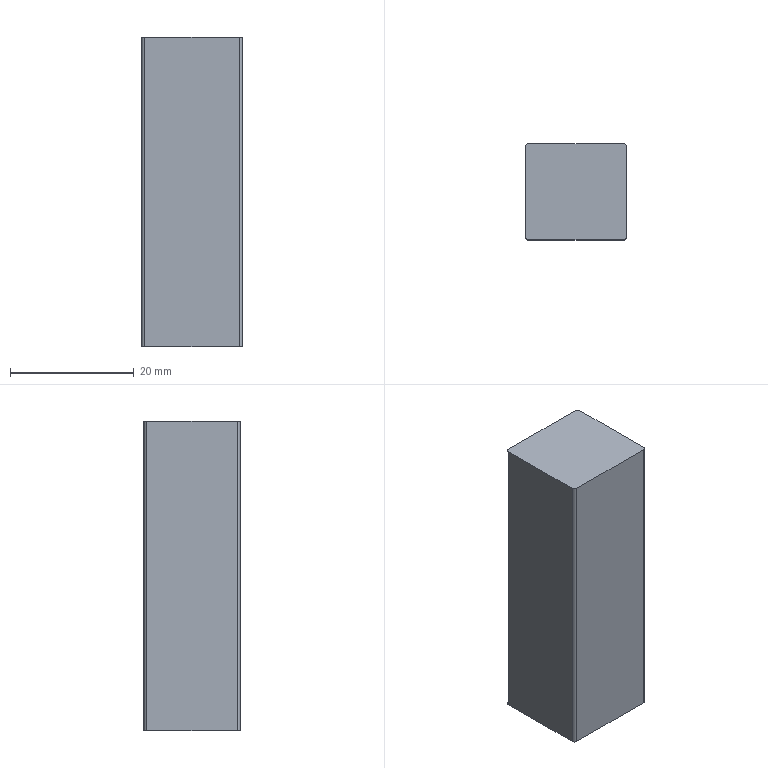Part | NX | features BREP 1 | 1 solid | 10 faces | box 16.274 x 15.522 x 50 mm | volume 12619 mm3 | plane 6 | cylinder 4 | commonest cylinder face diameters 1 x4
STEP:
#1=CARTESIAN_POINT('',(-7.637,7.761,-40.6));
#2=VERTEX_POINT('',#1);
#3=CARTESIAN_POINT('',(-8.137,7.261,-40.6));
#4=VERTEX_POINT('',#3);
#5=CARTESIAN_POINT('',(-7.637,7.261,-40.6));
#6=DIRECTION('',(0.,0.,1.));
#7=DIRECTION('',(1.,0.,0.));
#8=AXIS2_PLACEMENT_3D('',#5,#6,#7);
#9=CIRCLE('',#8,0.5);
#10=EDGE_CURVE('',#2,#4,#9,.T.);
#11=ORIENTED_EDGE('',*,*,#10,.F.);
#12=CARTESIAN_POINT('',(-7.637,7.761,-90.6));
#13=VERTEX_POINT('',#12);
#14=CARTESIAN_POINT('',(-7.637,7.761,-90.6));
#15=DIRECTION('',(0.,0.,1.));
#16=VECTOR('',#15,1000.);
#17=LINE('',#14,#16);
#18=EDGE_CURVE('',#13,#2,#17,.T.);
#19=ORIENTED_EDGE('',*,*,#18,.F.);
#20=CARTESIAN_POINT('',(-8.137,7.261,-90.6));
#21=VERTEX_POINT('',#20);
#22=CARTESIAN_POINT('',(-7.637,7.261,-90.6));
#23=DIRECTION('',(0.,0.,1.));
#24=DIRECTION('',(1.,0.,0.));
#25=AXIS2_PLACEMENT_3D('',#22,#23,#24);
#26=CIRCLE('',#25,0.5);
#27=EDGE_CURVE('',#13,#21,#26,.T.);
#28=ORIENTED_EDGE('',*,*,#27,.T.);
#29=CARTESIAN_POINT('',(-8.137,7.261,-90.6));
#30=DIRECTION('',(0.,0.,1.));
#31=VECTOR('',#30,1000.);
#32=LINE('',#29,#31);
#33=EDGE_CURVE('',#21,#4,#32,.T.);
#34=ORIENTED_EDGE('',*,*,#33,.T.);
#35=EDGE_LOOP('',(#11,#19,#28,#34));
#36=FACE_BOUND('',#35,.T.);
#37=CARTESIAN_POINT('',(-7.637,7.261,-90.6));
#38=DIRECTION('',(0.,0.,1.));
#39=DIRECTION('',(-1.,0.,0.));
#40=AXIS2_PLACEMENT_3D('',#37,#38,#39);
#41=CYLINDRICAL_SURFACE('',#40,0.5);
#42=ADVANCED_FACE('',(#36),#41,.T.);
#43=CARTESIAN_POINT('',(-8.137,-7.261,-40.6));
#44=VERTEX_POINT('',#43);
#45=CARTESIAN_POINT('',(-8.137,-7.261,-40.6));
#46=DIRECTION('',(0.,1.,0.));
#47=VECTOR('',#46,1000.);
#48=LINE('',#45,#47);
#49=EDGE_CURVE('',#44,#4,#48,.T.);
#50=ORIENTED_EDGE('',*,*,#49,.T.);
#51=ORIENTED_EDGE('',*,*,#33,.F.);
#52=CARTESIAN_POINT('',(-8.137,-7.261,-90.6));
#53=VERTEX_POINT('',#52);
#54=CARTESIAN_POINT('',(-8.137,-7.261,-90.6));
#55=DIRECTION('',(0.,1.,0.));
#56=VECTOR('',#55,1000.);
#57=LINE('',#54,#56);
#58=EDGE_CURVE('',#53,#21,#57,.T.);
#59=ORIENTED_EDGE('',*,*,#58,.F.);
#60=CARTESIAN_POINT('',(-8.137,-7.261,-90.6));
#61=DIRECTION('',(0.,0.,1.));
#62=VECTOR('',#61,1000.);
#63=LINE('',#60,#62);
#64=EDGE_CURVE('',#53,#44,#63,.T.);
#65=ORIENTED_EDGE('',*,*,#64,.T.);
#66=EDGE_LOOP('',(#50,#51,#59,#65));
#67=FACE_BOUND('',#66,.T.);
#68=CARTESIAN_POINT('',(-8.137,-7.261,-90.6));
#69=DIRECTION('',(1.,0.,0.));
#70=DIRECTION('',(0.,-1.,0.));
#71=AXIS2_PLACEMENT_3D('',#68,#69,#70);
#72=PLANE('',#71);
#73=ADVANCED_FACE('',(#67),#72,.F.);
#74=CARTESIAN_POINT('',(-7.637,-7.761,-40.6));
#75=VERTEX_POINT('',#74);
#76=CARTESIAN_POINT('',(-7.637,-7.261,-40.6));
#77=DIRECTION('',(0.,0.,1.));
#78=DIRECTION('',(1.,0.,0.));
#79=AXIS2_PLACEMENT_3D('',#76,#77,#78);
#80=CIRCLE('',#79,0.5);
#81=EDGE_CURVE('',#44,#75,#80,.T.);
#82=ORIENTED_EDGE('',*,*,#81,.F.);
#83=ORIENTED_EDGE('',*,*,#64,.F.);
#84=CARTESIAN_POINT('',(-7.637,-7.761,-90.6));
#85=VERTEX_POINT('',#84);
#86=CARTESIAN_POINT('',(-7.637,-7.261,-90.6));
#87=DIRECTION('',(0.,0.,1.));
#88=DIRECTION('',(1.,0.,0.));
#89=AXIS2_PLACEMENT_3D('',#86,#87,#88);
#90=CIRCLE('',#89,0.5);
#91=EDGE_CURVE('',#53,#85,#90,.T.);
#92=ORIENTED_EDGE('',*,*,#91,.T.);
#93=CARTESIAN_POINT('',(-7.637,-7.761,-90.6));
#94=DIRECTION('',(0.,0.,1.));
#95=VECTOR('',#94,1000.);
#96=LINE('',#93,#95);
#97=EDGE_CURVE('',#85,#75,#96,.T.);
#98=ORIENTED_EDGE('',*,*,#97,.T.);
#99=EDGE_LOOP('',(#82,#83,#92,#98));
#100=FACE_BOUND('',#99,.T.);
#101=CARTESIAN_POINT('',(-7.637,-7.261,-90.6));
#102=DIRECTION('',(0.,0.,1.));
#103=DIRECTION('',(-1.,0.,0.));
#104=AXIS2_PLACEMENT_3D('',#101,#102,#103);
#105=CYLINDRICAL_SURFACE('',#104,0.5);
#106=ADVANCED_FACE('',(#100),#105,.T.);
#107=CARTESIAN_POINT('',(7.637,-7.761,-40.6));
#108=VERTEX_POINT('',#107);
#109=CARTESIAN_POINT('',(7.637,-7.761,-40.6));
#110=DIRECTION('',(-1.,0.,0.));
#111=VECTOR('',#110,1000.);
#112=LINE('',#109,#111);
#113=EDGE_CURVE('',#108,#75,#112,.T.);
#114=ORIENTED_EDGE('',*,*,#113,.T.);
#115=ORIENTED_EDGE('',*,*,#97,.F.);
#116=CARTESIAN_POINT('',(7.637,-7.761,-90.6));
#117=VERTEX_POINT('',#116);
#118=CARTESIAN_POINT('',(7.637,-7.761,-90.6));
#119=DIRECTION('',(-1.,0.,0.));
#120=VECTOR('',#119,1000.);
#121=LINE('',#118,#120);
#122=EDGE_CURVE('',#117,#85,#121,.T.);
#123=ORIENTED_EDGE('',*,*,#122,.F.);
#124=CARTESIAN_POINT('',(7.637,-7.761,-90.6));
#125=DIRECTION('',(0.,0.,1.));
#126=VECTOR('',#125,1000.);
#127=LINE('',#124,#126);
#128=EDGE_CURVE('',#117,#108,#127,.T.);
#129=ORIENTED_EDGE('',*,*,#128,.T.);
#130=EDGE_LOOP('',(#114,#115,#123,#129));
#131=FACE_BOUND('',#130,.T.);
#132=CARTESIAN_POINT('',(7.637,-7.761,-90.6));
#133=DIRECTION('',(0.,1.,0.));
#134=DIRECTION('',(1.,0.,0.));
#135=AXIS2_PLACEMENT_3D('',#132,#133,#134);
#136=PLANE('',#135);
#137=ADVANCED_FACE('',(#131),#136,.F.);
#138=CARTESIAN_POINT('',(8.137,-7.261,-40.6));
#139=VERTEX_POINT('',#138);
#140=CARTESIAN_POINT('',(7.637,-7.261,-40.6));
#141=DIRECTION('',(0.,0.,1.));
#142=DIRECTION('',(1.,0.,0.));
#143=AXIS2_PLACEMENT_3D('',#140,#141,#142);
#144=CIRCLE('',#143,0.5);
#145=EDGE_CURVE('',#108,#139,#144,.T.);
#146=ORIENTED_EDGE('',*,*,#145,.F.);
#147=ORIENTED_EDGE('',*,*,#128,.F.);
#148=CARTESIAN_POINT('',(8.137,-7.261,-90.6));
#149=VERTEX_POINT('',#148);
#150=CARTESIAN_POINT('',(7.637,-7.261,-90.6));
#151=DIRECTION('',(0.,0.,1.));
#152=DIRECTION('',(1.,0.,0.));
#153=AXIS2_PLACEMENT_3D('',#150,#151,#152);
#154=CIRCLE('',#153,0.5);
#155=EDGE_CURVE('',#117,#149,#154,.T.);
#156=ORIENTED_EDGE('',*,*,#155,.T.);
#157=CARTESIAN_POINT('',(8.137,-7.261,-90.6));
#158=DIRECTION('',(0.,0.,1.));
#159=VECTOR('',#158,1000.);
#160=LINE('',#157,#159);
#161=EDGE_CURVE('',#149,#139,#160,.T.);
#162=ORIENTED_EDGE('',*,*,#161,.T.);
#163=EDGE_LOOP('',(#146,#147,#156,#162));
#164=FACE_BOUND('',#163,.T.);
#165=CARTESIAN_POINT('',(7.637,-7.261,-90.6));
#166=DIRECTION('',(0.,0.,1.));
#167=DIRECTION('',(-1.,0.,0.));
#168=AXIS2_PLACEMENT_3D('',#165,#166,#167);
#169=CYLINDRICAL_SURFACE('',#168,0.5);
#170=ADVANCED_FACE('',(#164),#169,.T.);
#171=CARTESIAN_POINT('',(8.137,7.261,-40.6));
#172=VERTEX_POINT('',#171);
#173=CARTESIAN_POINT('',(8.137,7.261,-40.6));
#174=DIRECTION('',(0.,-1.,0.));
#175=VECTOR('',#174,1000.);
#176=LINE('',#173,#175);
#177=EDGE_CURVE('',#172,#139,#176,.T.);
#178=ORIENTED_EDGE('',*,*,#177,.T.);
#179=ORIENTED_EDGE('',*,*,#161,.F.);
#180=CARTESIAN_POINT('',(8.137,7.261,-90.6));
#181=VERTEX_POINT('',#180);
#182=CARTESIAN_POINT('',(8.137,7.261,-90.6));
#183=DIRECTION('',(0.,-1.,0.));
#184=VECTOR('',#183,1000.);
#185=LINE('',#182,#184);
#186=EDGE_CURVE('',#181,#149,#185,.T.);
#187=ORIENTED_EDGE('',*,*,#186,.F.);
#188=CARTESIAN_POINT('',(8.137,7.261,-90.6));
#189=DIRECTION('',(0.,0.,1.));
#190=VECTOR('',#189,1000.);
#191=LINE('',#188,#190);
#192=EDGE_CURVE('',#181,#172,#191,.T.);
#193=ORIENTED_EDGE('',*,*,#192,.T.);
#194=EDGE_LOOP('',(#178,#179,#187,#193));
#195=FACE_BOUND('',#194,.T.);
#196=CARTESIAN_POINT('',(8.137,7.261,-90.6));
#197=DIRECTION('',(-1.,0.,0.));
#198=DIRECTION('',(0.,1.,0.));
#199=AXIS2_PLACEMENT_3D('',#196,#197,#198);
#200=PLANE('',#199);
#201=ADVANCED_FACE('',(#195),#200,.F.);
#202=CARTESIAN_POINT('',(7.637,7.761,-40.6));
#203=VERTEX_POINT('',#202);
#204=CARTESIAN_POINT('',(7.637,7.261,-40.6));
#205=DIRECTION('',(0.,0.,1.));
#206=DIRECTION('',(1.,0.,0.));
#207=AXIS2_PLACEMENT_3D('',#204,#205,#206);
#208=CIRCLE('',#207,0.5);
#209=EDGE_CURVE('',#172,#203,#208,.T.);
#210=ORIENTED_EDGE('',*,*,#209,.F.);
#211=ORIENTED_EDGE('',*,*,#192,.F.);
#212=CARTESIAN_POINT('',(7.637,7.761,-90.6));
#213=VERTEX_POINT('',#212);
#214=CARTESIAN_POINT('',(7.637,7.261,-90.6));
#215=DIRECTION('',(0.,0.,1.));
#216=DIRECTION('',(1.,0.,0.));
#217=AXIS2_PLACEMENT_3D('',#214,#215,#216);
#218=CIRCLE('',#217,0.5);
#219=EDGE_CURVE('',#181,#213,#218,.T.);
#220=ORIENTED_EDGE('',*,*,#219,.T.);
#221=CARTESIAN_POINT('',(7.637,7.761,-90.6));
#222=DIRECTION('',(0.,0.,1.));
#223=VECTOR('',#222,1000.);
#224=LINE('',#221,#223);
#225=EDGE_CURVE('',#213,#203,#224,.T.);
#226=ORIENTED_EDGE('',*,*,#225,.T.);
#227=EDGE_LOOP('',(#210,#211,#220,#226));
#228=FACE_BOUND('',#227,.T.);
#229=CARTESIAN_POINT('',(7.637,7.261,-90.6));
#230=DIRECTION('',(0.,0.,1.));
#231=DIRECTION('',(-1.,0.,0.));
#232=AXIS2_PLACEMENT_3D('',#229,#230,#231);
#233=CYLINDRICAL_SURFACE('',#232,0.5);
#234=ADVANCED_FACE('',(#228),#233,.T.);
#235=CARTESIAN_POINT('',(-7.637,7.761,-40.6));
#236=DIRECTION('',(1.,0.,0.));
#237=VECTOR('',#236,1000.);
#238=LINE('',#235,#237);
#239=EDGE_CURVE('',#2,#203,#238,.T.);
#240=ORIENTED_EDGE('',*,*,#239,.T.);
#241=ORIENTED_EDGE('',*,*,#225,.F.);
#242=CARTESIAN_POINT('',(-7.637,7.761,-90.6));
#243=DIRECTION('',(1.,0.,0.));
#244=VECTOR('',#243,1000.);
#245=LINE('',#242,#244);
#246=EDGE_CURVE('',#13,#213,#245,.T.);
#247=ORIENTED_EDGE('',*,*,#246,.F.);
#248=ORIENTED_EDGE('',*,*,#18,.T.);
#249=EDGE_LOOP('',(#240,#241,#247,#248));
#250=FACE_BOUND('',#249,.T.);
#251=CARTESIAN_POINT('',(-7.637,7.761,-90.6));
#252=DIRECTION('',(0.,-1.,0.));
#253=DIRECTION('',(0.,0.,1.));
#254=AXIS2_PLACEMENT_3D('',#251,#252,#253);
#255=PLANE('',#254);
#256=ADVANCED_FACE('',(#250),#255,.F.);
#257=ORIENTED_EDGE('',*,*,#27,.F.);
#258=ORIENTED_EDGE('',*,*,#246,.T.);
#259=ORIENTED_EDGE('',*,*,#219,.F.);
#260=ORIENTED_EDGE('',*,*,#186,.T.);
#261=ORIENTED_EDGE('',*,*,#155,.F.);
#262=ORIENTED_EDGE('',*,*,#122,.T.);
#263=ORIENTED_EDGE('',*,*,#91,.F.);
#264=ORIENTED_EDGE('',*,*,#58,.T.);
#265=EDGE_LOOP('',(#257,#258,#259,#260,#261,#262,#263,#264));
#266=FACE_BOUND('',#265,.T.);
#267=CARTESIAN_POINT('',(-7.637,7.261,-90.6));
#268=DIRECTION('',(0.,0.,1.));
#269=DIRECTION('',(-1.,0.,0.));
#270=AXIS2_PLACEMENT_3D('',#267,#268,#269);
#271=PLANE('',#270);
#272=ADVANCED_FACE('',(#266),#271,.F.);
#273=ORIENTED_EDGE('',*,*,#10,.T.);
#274=ORIENTED_EDGE('',*,*,#49,.F.);
#275=ORIENTED_EDGE('',*,*,#81,.T.);
#276=ORIENTED_EDGE('',*,*,#113,.F.);
#277=ORIENTED_EDGE('',*,*,#145,.T.);
#278=ORIENTED_EDGE('',*,*,#177,.F.);
#279=ORIENTED_EDGE('',*,*,#209,.T.);
#280=ORIENTED_EDGE('',*,*,#239,.F.);
#281=EDGE_LOOP('',(#273,#274,#275,#276,#277,#278,#279,#280));
#282=FACE_BOUND('',#281,.T.);
#283=CARTESIAN_POINT('',(-7.637,7.261,-40.6));
#284=DIRECTION('',(0.,0.,1.));
#285=DIRECTION('',(-1.,0.,0.));
#286=AXIS2_PLACEMENT_3D('',#283,#284,#285);
#287=PLANE('',#286);
#288=ADVANCED_FACE('',(#282),#287,.T.);
#289=CLOSED_SHELL('',(#42,#73,#106,#137,#170,#201,#234,#256,#272,#288));
#290=MANIFOLD_SOLID_BREP('',#289);
#291=(LENGTH_UNIT()NAMED_UNIT(*)SI_UNIT(.MILLI.,.METRE.));
#292=UNCERTAINTY_MEASURE_WITH_UNIT(LENGTH_MEASURE(0.00001),#291,'','');
#293=(NAMED_UNIT(*)PLANE_ANGLE_UNIT()SI_UNIT($,.RADIAN.));
#294=(NAMED_UNIT(*)SI_UNIT($,.STERADIAN.)SOLID_ANGLE_UNIT());
#295=(GEOMETRIC_REPRESENTATION_CONTEXT(3)GLOBAL_UNCERTAINTY_ASSIGNED_CONTEXT((#292))GLOBAL_UNIT_ASSIGNED_CONTEXT((#291,#293,#294))REPRESENTATION_CONTEXT('',''));
#296=ADVANCED_BREP_SHAPE_REPRESENTATION('',(#290),#295);